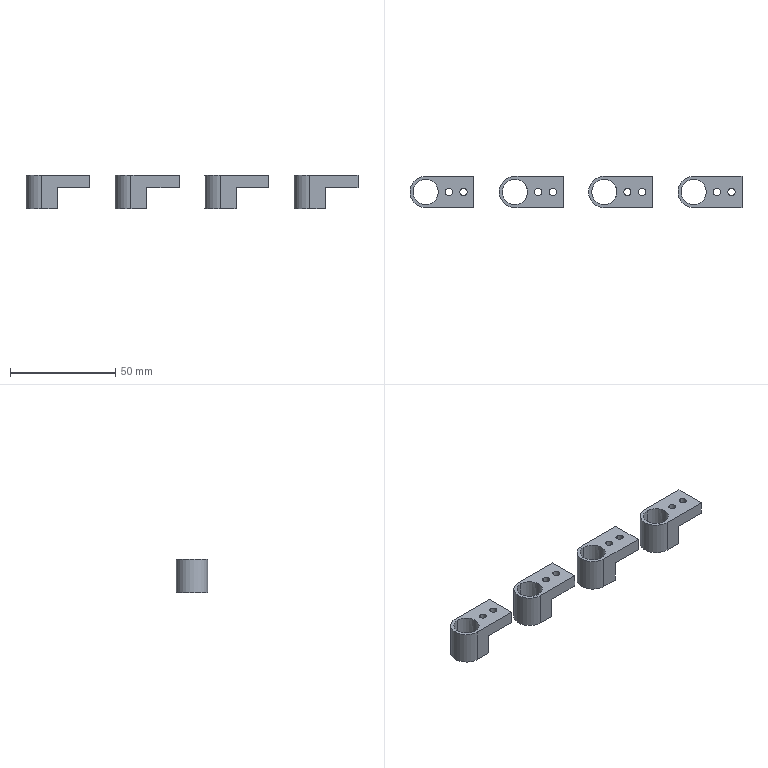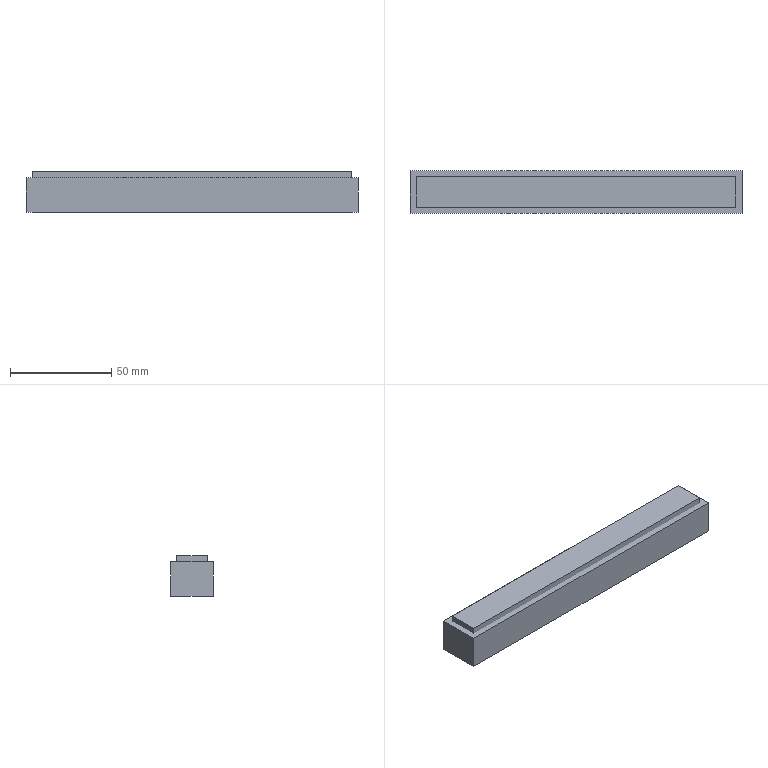CAM job | NX | 3-axis milling, drilling | part box 158 x 15 x 16 mm | stock box 164 x 21 x 20 mm
Tools:
number,name,description,diameter,corner_radius,flute_length,length,flutes
3,D63,Milling Tool-5 Parameters,63.0,0.0,50.0,75.0,2
1,D6A45,Milling Tool-5 Parameters,6.0,0.0,3.0,3.0,2
13,3.4ZT,Drilling Tool,3.4,0.0,35.0,50.0,2
4,D10,Milling Tool-5 Parameters,10.0,0.0,50.0,75.0,2
14,D10JING,Milling Tool-5 Parameters,10.0,0.0,50.0,75.0,2
Operations:
program,operation,operation_type,tool,method,geometry_group,spindle_rpm,surface_speed,feed_per_tooth,feed_cut,feed_plunge,cut_length_mm,path_length_mm,cut_time_min,machine_time_min
1,FLOOR_WALL,VolumeBased25DMillingOperation,D63,METHOD,A,6500.0,1286.0,0.1154,1500.0,100.0,239.0,293.0,0.1593,0.1647
1,DRILLING,Operation,D6A45,METHOD,A,5000.0,94.0,0.025,250.0,0.0,48.0,339.119,0.192,0.2211
1,DRILLING_COPY,Operation,3.4ZT,METHOD,A,2000.0,21.0,0.0375,150.0,0.0,133.693,457.805,0.8913,0.9237
1,ZLEVEL_PROFILE_1,ZLevelMilling,D10,METHOD,A,7500.0,235.0,0.2,3000.0,1000.0,7889.472,8343.525,2.757,2.803
1,HOLE_MILLING_COPY,CylinderMilling,D10,METHOD,A,7500.0,235.0,0.1467,2200.0,100.0,505.101,934.601,0.2296,0.2725
1,ZLEVEL_PROFILE,ZLevelMilling,D10JING,METHOD,A,7500.0,235.0,0.0667,1000.0,100.0,493.697,970.973,0.4937,0.5414
1,PLANAR_MILL,PlanarMilling,D6A45,METHOD,A,7500.0,141.0,0.0833,1250.0,100.0,614.201,1728.569,0.4914,0.6028
1,刀补14,CylinderMilling,D10JING,METHOD,A,7500.0,235.0,0.0667,1000.0,100.0,243.637,673.137,0.2436,0.2866
2,FLOOR_WALL_COPY,VolumeBased25DMillingOperation,D63,METHOD,B,6500.0,1286.0,0.1154,1500.0,100.0,932.0,1817.001,0.6213,0.7098
2,FLOOR_WALL_1,VolumeBased25DMillingOperation,D10,METHOD,B,7500.0,235.0,0.1667,2500.0,1000.0,2188.2,2565.75,0.8897,0.9274
2,FLOOR_WALL_1_COPY,VolumeBased25DMillingOperation,D10JING,METHOD,B,7500.0,235.0,0.08,1200.0,1000.0,535.988,1385.671,0.4547,0.5396
2,ZLEVEL_PROFILE_2,ZLevelMilling,D6A45,METHOD,B,7500.0,141.0,0.0833,1250.0,100.0,446.384,1170.062,0.3571,0.4295
2,ZLEVEL_PROFILE_2_COPY,ZLevelMilling,D6A45,METHOD,B,7500.0,141.0,0.0833,1250.0,100.0,291.024,1831.869,0.2328,0.3869